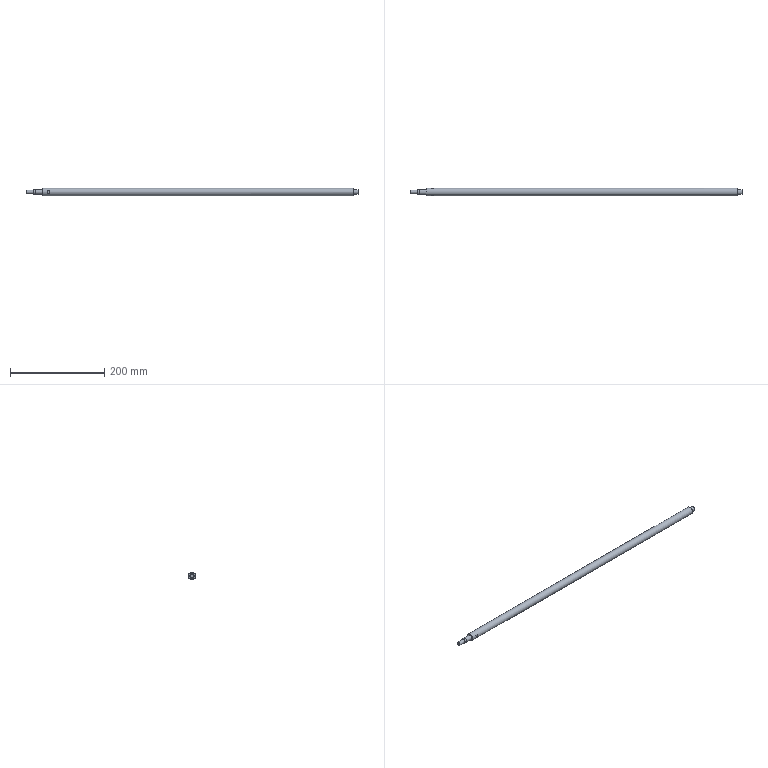Part | NX | 1 solid | 17 faces | box 705 x 16 x 16 mm | volume 135751 mm3 | plane 12 | cylinder 5 | commonest cylinder face diameters 10 x2 8 x1 9.9 x1 16 x1
STEP:
#1=CARTESIAN_POINT('',(50.,-7.,-3.873));
#2=VERTEX_POINT('',#1);
#3=CARTESIAN_POINT('',(50.,-7.,3.873));
#4=VERTEX_POINT('',#3);
#5=CARTESIAN_POINT('',(50.,0.,0.));
#6=DIRECTION('',(-1.,0.,0.));
#7=DIRECTION('',(0.,0.,-1.));
#8=AXIS2_PLACEMENT_3D('',#5,#6,#7);
#9=CIRCLE('',#8,8.);
#10=EDGE_CURVE('',#2,#4,#9,.T.);
#11=ORIENTED_EDGE('',*,*,#10,.F.);
#12=CARTESIAN_POINT('',(45.,-7.,-3.873));
#13=VERTEX_POINT('',#12);
#14=CARTESIAN_POINT('',(355.,-7.,-3.873));
#15=DIRECTION('',(1.,0.,0.));
#16=VECTOR('',#15,1.);
#17=LINE('',#14,#16);
#18=EDGE_CURVE('',#13,#2,#17,.T.);
#19=ORIENTED_EDGE('',*,*,#18,.F.);
#20=CARTESIAN_POINT('',(45.,-7.,3.873));
#21=VERTEX_POINT('',#20);
#22=CARTESIAN_POINT('',(45.,0.,0.));
#23=DIRECTION('',(1.,0.,0.));
#24=DIRECTION('',(0.,0.,1.));
#25=AXIS2_PLACEMENT_3D('',#22,#23,#24);
#26=CIRCLE('',#25,8.);
#27=EDGE_CURVE('',#21,#13,#26,.T.);
#28=ORIENTED_EDGE('',*,*,#27,.F.);
#29=CARTESIAN_POINT('',(355.,-7.,3.873));
#30=DIRECTION('',(-1.,0.,0.));
#31=VECTOR('',#30,1.);
#32=LINE('',#29,#31);
#33=EDGE_CURVE('',#4,#21,#32,.T.);
#34=ORIENTED_EDGE('',*,*,#33,.F.);
#35=EDGE_LOOP('',(#11,#19,#28,#34));
#36=FACE_BOUND('',#35,.T.);
#37=CARTESIAN_POINT('',(695.,0.,8.));
#38=VERTEX_POINT('',#37);
#39=CARTESIAN_POINT('',(695.,0.,0.));
#40=DIRECTION('',(-1.,0.,0.));
#41=DIRECTION('',(0.,0.,1.));
#42=AXIS2_PLACEMENT_3D('',#39,#40,#41);
#43=CIRCLE('',#42,8.);
#44=EDGE_CURVE('',#38,#38,#43,.T.);
#45=ORIENTED_EDGE('',*,*,#44,.T.);
#46=EDGE_LOOP('',(#45));
#47=FACE_BOUND('',#46,.T.);
#48=CARTESIAN_POINT('',(35.,0.,8.));
#49=VERTEX_POINT('',#48);
#50=CARTESIAN_POINT('',(35.,0.,0.));
#51=DIRECTION('',(-1.,0.,0.));
#52=DIRECTION('',(0.,0.,1.));
#53=AXIS2_PLACEMENT_3D('',#50,#51,#52);
#54=CIRCLE('',#53,8.);
#55=EDGE_CURVE('',#49,#49,#54,.T.);
#56=ORIENTED_EDGE('',*,*,#55,.F.);
#57=EDGE_LOOP('',(#56));
#58=FACE_BOUND('',#57,.T.);
#59=CARTESIAN_POINT('',(45.,7.,-3.873));
#60=VERTEX_POINT('',#59);
#61=CARTESIAN_POINT('',(50.,7.,-3.873));
#62=VERTEX_POINT('',#61);
#63=CARTESIAN_POINT('',(355.,7.,-3.873));
#64=DIRECTION('',(1.,0.,0.));
#65=VECTOR('',#64,1.);
#66=LINE('',#63,#65);
#67=EDGE_CURVE('',#60,#62,#66,.T.);
#68=ORIENTED_EDGE('',*,*,#67,.T.);
#69=CARTESIAN_POINT('',(50.,7.,3.873));
#70=VERTEX_POINT('',#69);
#71=CARTESIAN_POINT('',(50.,0.,0.));
#72=DIRECTION('',(1.,0.,0.));
#73=DIRECTION('',(0.,0.,1.));
#74=AXIS2_PLACEMENT_3D('',#71,#72,#73);
#75=CIRCLE('',#74,8.);
#76=EDGE_CURVE('',#62,#70,#75,.T.);
#77=ORIENTED_EDGE('',*,*,#76,.T.);
#78=CARTESIAN_POINT('',(45.,7.,3.873));
#79=VERTEX_POINT('',#78);
#80=CARTESIAN_POINT('',(355.,7.,3.873));
#81=DIRECTION('',(-1.,0.,0.));
#82=VECTOR('',#81,1.);
#83=LINE('',#80,#82);
#84=EDGE_CURVE('',#70,#79,#83,.T.);
#85=ORIENTED_EDGE('',*,*,#84,.T.);
#86=CARTESIAN_POINT('',(45.,0.,0.));
#87=DIRECTION('',(-1.,0.,0.));
#88=DIRECTION('',(0.,0.,-1.));
#89=AXIS2_PLACEMENT_3D('',#86,#87,#88);
#90=CIRCLE('',#89,8.);
#91=EDGE_CURVE('',#79,#60,#90,.T.);
#92=ORIENTED_EDGE('',*,*,#91,.T.);
#93=EDGE_LOOP('',(#68,#77,#85,#92));
#94=FACE_BOUND('',#93,.T.);
#95=CARTESIAN_POINT('',(355.,0.,0.));
#96=DIRECTION('',(-1.,0.,0.));
#97=DIRECTION('',(0.,0.,-1.));
#98=AXIS2_PLACEMENT_3D('',#95,#96,#97);
#99=CYLINDRICAL_SURFACE('',#98,8.);
#100=ADVANCED_FACE('',(#36,#47,#58,#94),#99,.T.);
#101=CARTESIAN_POINT('',(0.,0.,4.));
#102=VERTEX_POINT('',#101);
#103=CARTESIAN_POINT('',(0.,0.,0.));
#104=DIRECTION('',(-1.,0.,0.));
#105=DIRECTION('',(0.,0.,1.));
#106=AXIS2_PLACEMENT_3D('',#103,#104,#105);
#107=CIRCLE('',#106,4.);
#108=EDGE_CURVE('',#102,#102,#107,.T.);
#109=ORIENTED_EDGE('',*,*,#108,.T.);
#110=EDGE_LOOP('',(#109));
#111=FACE_OUTER_BOUND('',#110,.T.);
#112=CARTESIAN_POINT('',(0.,0.,0.));
#113=DIRECTION('',(-1.,0.,0.));
#114=DIRECTION('',(0.,0.,-1.));
#115=AXIS2_PLACEMENT_3D('',#112,#113,#114);
#116=PLANE('',#115);
#117=ADVANCED_FACE('',(#111),#116,.T.);
#118=CARTESIAN_POINT('',(15.,0.,4.));
#119=VERTEX_POINT('',#118);
#120=CARTESIAN_POINT('',(15.,0.,0.));
#121=DIRECTION('',(-1.,0.,0.));
#122=DIRECTION('',(0.,0.,1.));
#123=AXIS2_PLACEMENT_3D('',#120,#121,#122);
#124=CIRCLE('',#123,4.);
#125=EDGE_CURVE('',#119,#119,#124,.T.);
#126=ORIENTED_EDGE('',*,*,#125,.T.);
#127=EDGE_LOOP('',(#126));
#128=FACE_BOUND('',#127,.T.);
#129=ORIENTED_EDGE('',*,*,#108,.F.);
#130=EDGE_LOOP('',(#129));
#131=FACE_BOUND('',#130,.T.);
#132=CARTESIAN_POINT('',(355.,0.,0.));
#133=DIRECTION('',(-1.,0.,0.));
#134=DIRECTION('',(0.,0.,-1.));
#135=AXIS2_PLACEMENT_3D('',#132,#133,#134);
#136=CYLINDRICAL_SURFACE('',#135,4.);
#137=ADVANCED_FACE('',(#128,#131),#136,.T.);
#138=CARTESIAN_POINT('',(15.,0.,4.95));
#139=VERTEX_POINT('',#138);
#140=CARTESIAN_POINT('',(15.,0.,0.));
#141=DIRECTION('',(-1.,0.,0.));
#142=DIRECTION('',(0.,0.,1.));
#143=AXIS2_PLACEMENT_3D('',#140,#141,#142);
#144=CIRCLE('',#143,4.95);
#145=EDGE_CURVE('',#139,#139,#144,.T.);
#146=ORIENTED_EDGE('',*,*,#145,.T.);
#147=EDGE_LOOP('',(#146));
#148=FACE_BOUND('',#147,.T.);
#149=ORIENTED_EDGE('',*,*,#125,.F.);
#150=EDGE_LOOP('',(#149));
#151=FACE_BOUND('',#150,.T.);
#152=CARTESIAN_POINT('',(15.,0.,4.));
#153=DIRECTION('',(-1.,0.,0.));
#154=DIRECTION('',(0.,0.,-1.));
#155=AXIS2_PLACEMENT_3D('',#152,#153,#154);
#156=PLANE('',#155);
#157=ADVANCED_FACE('',(#148,#151),#156,.T.);
#158=CARTESIAN_POINT('',(20.,0.,4.95));
#159=VERTEX_POINT('',#158);
#160=CARTESIAN_POINT('',(20.,0.,0.));
#161=DIRECTION('',(-1.,0.,0.));
#162=DIRECTION('',(0.,0.,1.));
#163=AXIS2_PLACEMENT_3D('',#160,#161,#162);
#164=CIRCLE('',#163,4.95);
#165=EDGE_CURVE('',#159,#159,#164,.T.);
#166=ORIENTED_EDGE('',*,*,#165,.T.);
#167=EDGE_LOOP('',(#166));
#168=FACE_BOUND('',#167,.T.);
#169=ORIENTED_EDGE('',*,*,#145,.F.);
#170=EDGE_LOOP('',(#169));
#171=FACE_BOUND('',#170,.T.);
#172=CARTESIAN_POINT('',(355.,0.,0.));
#173=DIRECTION('',(-1.,0.,0.));
#174=DIRECTION('',(0.,0.,-1.));
#175=AXIS2_PLACEMENT_3D('',#172,#173,#174);
#176=CYLINDRICAL_SURFACE('',#175,4.95);
#177=ADVANCED_FACE('',(#168,#171),#176,.T.);
#178=CARTESIAN_POINT('',(20.,0.,5.));
#179=VERTEX_POINT('',#178);
#180=CARTESIAN_POINT('',(20.,0.,0.));
#181=DIRECTION('',(-1.,0.,0.));
#182=DIRECTION('',(0.,0.,1.));
#183=AXIS2_PLACEMENT_3D('',#180,#181,#182);
#184=CIRCLE('',#183,5.);
#185=EDGE_CURVE('',#179,#179,#184,.T.);
#186=ORIENTED_EDGE('',*,*,#185,.T.);
#187=EDGE_LOOP('',(#186));
#188=FACE_BOUND('',#187,.T.);
#189=ORIENTED_EDGE('',*,*,#165,.F.);
#190=EDGE_LOOP('',(#189));
#191=FACE_BOUND('',#190,.T.);
#192=CARTESIAN_POINT('',(20.,0.,4.95));
#193=DIRECTION('',(-1.,0.,0.));
#194=DIRECTION('',(0.,0.,-1.));
#195=AXIS2_PLACEMENT_3D('',#192,#193,#194);
#196=PLANE('',#195);
#197=ADVANCED_FACE('',(#188,#191),#196,.T.);
#198=CARTESIAN_POINT('',(35.,0.,5.));
#199=VERTEX_POINT('',#198);
#200=CARTESIAN_POINT('',(35.,0.,0.));
#201=DIRECTION('',(-1.,0.,0.));
#202=DIRECTION('',(0.,0.,1.));
#203=AXIS2_PLACEMENT_3D('',#200,#201,#202);
#204=CIRCLE('',#203,5.);
#205=EDGE_CURVE('',#199,#199,#204,.T.);
#206=ORIENTED_EDGE('',*,*,#205,.T.);
#207=EDGE_LOOP('',(#206));
#208=FACE_BOUND('',#207,.T.);
#209=ORIENTED_EDGE('',*,*,#185,.F.);
#210=EDGE_LOOP('',(#209));
#211=FACE_BOUND('',#210,.T.);
#212=CARTESIAN_POINT('',(355.,0.,0.));
#213=DIRECTION('',(-1.,0.,0.));
#214=DIRECTION('',(0.,0.,-1.));
#215=AXIS2_PLACEMENT_3D('',#212,#213,#214);
#216=CYLINDRICAL_SURFACE('',#215,5.);
#217=ADVANCED_FACE('',(#208,#211),#216,.T.);
#218=ORIENTED_EDGE('',*,*,#55,.T.);
#219=EDGE_LOOP('',(#218));
#220=FACE_BOUND('',#219,.T.);
#221=ORIENTED_EDGE('',*,*,#205,.F.);
#222=EDGE_LOOP('',(#221));
#223=FACE_BOUND('',#222,.T.);
#224=CARTESIAN_POINT('',(35.,0.,5.));
#225=DIRECTION('',(-1.,0.,0.));
#226=DIRECTION('',(0.,0.,-1.));
#227=AXIS2_PLACEMENT_3D('',#224,#225,#226);
#228=PLANE('',#227);
#229=ADVANCED_FACE('',(#220,#223),#228,.T.);
#230=CARTESIAN_POINT('',(695.,0.,5.));
#231=VERTEX_POINT('',#230);
#232=CARTESIAN_POINT('',(695.,0.,0.));
#233=DIRECTION('',(-1.,0.,0.));
#234=DIRECTION('',(0.,0.,1.));
#235=AXIS2_PLACEMENT_3D('',#232,#233,#234);
#236=CIRCLE('',#235,5.);
#237=EDGE_CURVE('',#231,#231,#236,.T.);
#238=ORIENTED_EDGE('',*,*,#237,.T.);
#239=EDGE_LOOP('',(#238));
#240=FACE_BOUND('',#239,.T.);
#241=ORIENTED_EDGE('',*,*,#44,.F.);
#242=EDGE_LOOP('',(#241));
#243=FACE_BOUND('',#242,.T.);
#244=CARTESIAN_POINT('',(695.,0.,8.));
#245=DIRECTION('',(1.,0.,0.));
#246=DIRECTION('',(0.,0.,1.));
#247=AXIS2_PLACEMENT_3D('',#244,#245,#246);
#248=PLANE('',#247);
#249=ADVANCED_FACE('',(#240,#243),#248,.T.);
#250=CARTESIAN_POINT('',(705.,0.,5.));
#251=VERTEX_POINT('',#250);
#252=CARTESIAN_POINT('',(705.,0.,0.));
#253=DIRECTION('',(-1.,0.,0.));
#254=DIRECTION('',(0.,0.,1.));
#255=AXIS2_PLACEMENT_3D('',#252,#253,#254);
#256=CIRCLE('',#255,5.);
#257=EDGE_CURVE('',#251,#251,#256,.T.);
#258=ORIENTED_EDGE('',*,*,#257,.T.);
#259=EDGE_LOOP('',(#258));
#260=FACE_BOUND('',#259,.T.);
#261=ORIENTED_EDGE('',*,*,#237,.F.);
#262=EDGE_LOOP('',(#261));
#263=FACE_BOUND('',#262,.T.);
#264=CARTESIAN_POINT('',(705.,0.,0.));
#265=DIRECTION('',(-1.,0.,0.));
#266=DIRECTION('',(0.,0.,-1.));
#267=AXIS2_PLACEMENT_3D('',#264,#265,#266);
#268=CYLINDRICAL_SURFACE('',#267,5.);
#269=ADVANCED_FACE('',(#260,#263),#268,.T.);
#270=ORIENTED_EDGE('',*,*,#257,.F.);
#271=EDGE_LOOP('',(#270));
#272=FACE_OUTER_BOUND('',#271,.T.);
#273=CARTESIAN_POINT('',(705.,0.,5.));
#274=DIRECTION('',(1.,0.,0.));
#275=DIRECTION('',(0.,0.,1.));
#276=AXIS2_PLACEMENT_3D('',#273,#274,#275);
#277=PLANE('',#276);
#278=ADVANCED_FACE('',(#272),#277,.T.);
#279=CARTESIAN_POINT('',(45.,7.,20.));
#280=DIRECTION('',(0.,0.,1.));
#281=VECTOR('',#280,1.);
#282=LINE('',#279,#281);
#283=EDGE_CURVE('',#60,#79,#282,.T.);
#284=ORIENTED_EDGE('',*,*,#283,.F.);
#285=ORIENTED_EDGE('',*,*,#91,.F.);
#286=EDGE_LOOP('',(#284,#285));
#287=FACE_OUTER_BOUND('',#286,.T.);
#288=CARTESIAN_POINT('',(45.,8.,20.));
#289=DIRECTION('',(1.,0.,0.));
#290=DIRECTION('',(0.,0.,1.));
#291=AXIS2_PLACEMENT_3D('',#288,#289,#290);
#292=PLANE('',#291);
#293=ADVANCED_FACE('',(#287),#292,.T.);
#294=ORIENTED_EDGE('',*,*,#283,.T.);
#295=ORIENTED_EDGE('',*,*,#84,.F.);
#296=CARTESIAN_POINT('',(50.,7.,20.));
#297=DIRECTION('',(0.,0.,1.));
#298=VECTOR('',#297,1.);
#299=LINE('',#296,#298);
#300=EDGE_CURVE('',#62,#70,#299,.T.);
#301=ORIENTED_EDGE('',*,*,#300,.F.);
#302=ORIENTED_EDGE('',*,*,#67,.F.);
#303=EDGE_LOOP('',(#294,#295,#301,#302));
#304=FACE_OUTER_BOUND('',#303,.T.);
#305=CARTESIAN_POINT('',(45.,7.,20.));
#306=DIRECTION('',(0.,1.,0.));
#307=DIRECTION('',(0.,0.,-1.));
#308=AXIS2_PLACEMENT_3D('',#305,#306,#307);
#309=PLANE('',#308);
#310=ADVANCED_FACE('',(#304),#309,.T.);
#311=ORIENTED_EDGE('',*,*,#300,.T.);
#312=ORIENTED_EDGE('',*,*,#76,.F.);
#313=EDGE_LOOP('',(#311,#312));
#314=FACE_OUTER_BOUND('',#313,.T.);
#315=CARTESIAN_POINT('',(50.,7.,20.));
#316=DIRECTION('',(-1.,0.,0.));
#317=DIRECTION('',(0.,0.,-1.));
#318=AXIS2_PLACEMENT_3D('',#315,#316,#317);
#319=PLANE('',#318);
#320=ADVANCED_FACE('',(#314),#319,.T.);
#321=CARTESIAN_POINT('',(45.,-7.,20.));
#322=DIRECTION('',(0.,0.,1.));
#323=VECTOR('',#322,1.);
#324=LINE('',#321,#323);
#325=EDGE_CURVE('',#13,#21,#324,.T.);
#326=ORIENTED_EDGE('',*,*,#325,.T.);
#327=ORIENTED_EDGE('',*,*,#27,.T.);
#328=EDGE_LOOP('',(#326,#327));
#329=FACE_OUTER_BOUND('',#328,.T.);
#330=CARTESIAN_POINT('',(45.,-8.,20.));
#331=DIRECTION('',(-1.,0.,0.));
#332=DIRECTION('',(0.,0.,-1.));
#333=AXIS2_PLACEMENT_3D('',#330,#331,#332);
#334=PLANE('',#333);
#335=ADVANCED_FACE('',(#329),#334,.F.);
#336=ORIENTED_EDGE('',*,*,#18,.T.);
#337=CARTESIAN_POINT('',(50.,-7.,20.));
#338=DIRECTION('',(0.,0.,1.));
#339=VECTOR('',#338,1.);
#340=LINE('',#337,#339);
#341=EDGE_CURVE('',#2,#4,#340,.T.);
#342=ORIENTED_EDGE('',*,*,#341,.T.);
#343=ORIENTED_EDGE('',*,*,#33,.T.);
#344=ORIENTED_EDGE('',*,*,#325,.F.);
#345=EDGE_LOOP('',(#336,#342,#343,#344));
#346=FACE_OUTER_BOUND('',#345,.T.);
#347=CARTESIAN_POINT('',(45.,-7.,20.));
#348=DIRECTION('',(0.,1.,0.));
#349=DIRECTION('',(0.,0.,-1.));
#350=AXIS2_PLACEMENT_3D('',#347,#348,#349);
#351=PLANE('',#350);
#352=ADVANCED_FACE('',(#346),#351,.F.);
#353=ORIENTED_EDGE('',*,*,#341,.F.);
#354=ORIENTED_EDGE('',*,*,#10,.T.);
#355=EDGE_LOOP('',(#353,#354));
#356=FACE_OUTER_BOUND('',#355,.T.);
#357=CARTESIAN_POINT('',(50.,-7.,20.));
#358=DIRECTION('',(1.,0.,0.));
#359=DIRECTION('',(0.,0.,1.));
#360=AXIS2_PLACEMENT_3D('',#357,#358,#359);
#361=PLANE('',#360);
#362=ADVANCED_FACE('',(#356),#361,.F.);
#363=CLOSED_SHELL('',(#100,#117,#137,#157,#177,#197,#217,#229,#249,#269,#278,#293,#310,#320,#335,#352,#362));
#364=MANIFOLD_SOLID_BREP('',#363);
#365=(LENGTH_UNIT()NAMED_UNIT(*)SI_UNIT(.MILLI.,.METRE.));
#366=UNCERTAINTY_MEASURE_WITH_UNIT(LENGTH_MEASURE(0.00002),#365,'','');
#367=(NAMED_UNIT(*)PLANE_ANGLE_UNIT()SI_UNIT($,.RADIAN.));
#368=PLANE_ANGLE_MEASURE_WITH_UNIT(PLANE_ANGLE_MEASURE(0.01745),#367);
#369=DIMENSIONAL_EXPONENTS(0.,0.,0.,0.,0.,0.,0.);
#370=(CONVERSION_BASED_UNIT('DEGREE',#368)NAMED_UNIT(#369)PLANE_ANGLE_UNIT());
#371=(NAMED_UNIT(*)SI_UNIT($,.STERADIAN.)SOLID_ANGLE_UNIT());
#372=(GEOMETRIC_REPRESENTATION_CONTEXT(3)GLOBAL_UNCERTAINTY_ASSIGNED_CONTEXT((#366))GLOBAL_UNIT_ASSIGNED_CONTEXT((#365,#370,#371))REPRESENTATION_CONTEXT('',''));
#373=ADVANCED_BREP_SHAPE_REPRESENTATION('',(#364),#372);